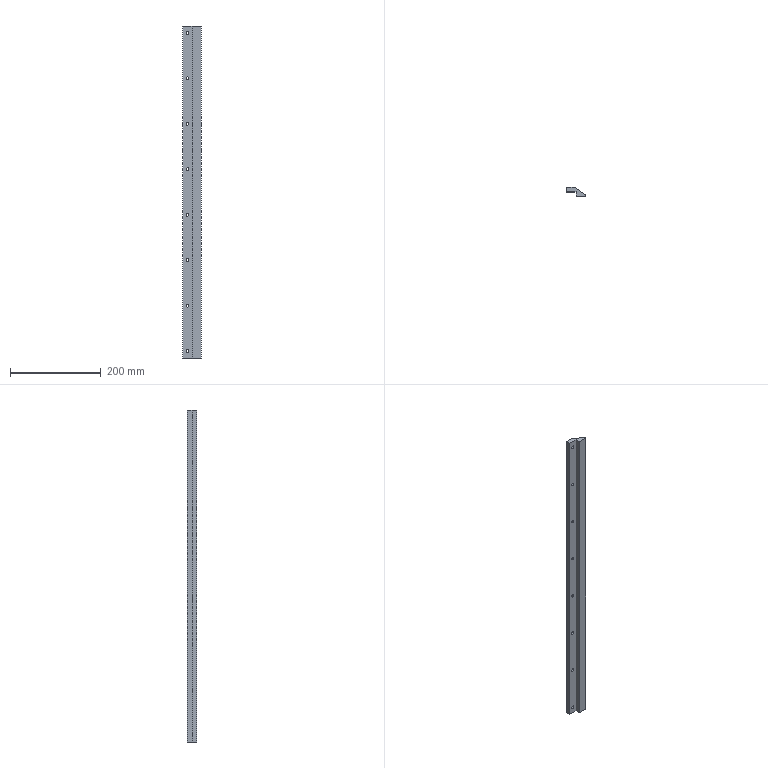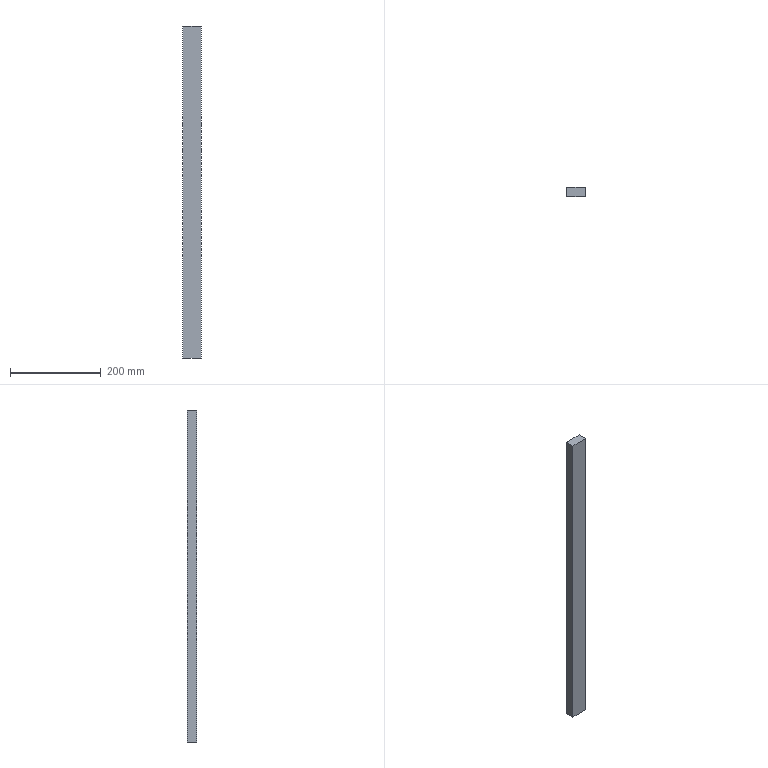CAM job | NX | 3+2 milling, drilling | part box 40 x 20 x 730 mm | stock box 40 x 20 x 730 mm
Tools:
number,name,description,diameter,corner_radius,flute_length,length,flutes
15,D10,Milling Tool-5 Parameters,10.0,0.0,50.0,75.0,2
14,D10JING,Milling Tool-5 Parameters,10.0,0.0,50.0,75.0,2
1,D6A45,Milling Tool-5 Parameters,6.0,0.0,50.0,75.0,2
16,6.2ZT,Drilling Tool,6.2,0.0,35.0,50.0,2
16,D6R0.5,Milling Tool-5 Parameters,6.0,0.5,50.0,75.0,2
Operations:
program,operation,operation_type,tool,method,geometry_group,spindle_rpm,surface_speed,feed_per_tooth,feed_cut,feed_plunge,cut_length_mm,path_length_mm,cut_time_min,machine_time_min
1,FLOOR_WALL_1,VolumeBased25DMillingOperation,D10,METHOD,A,9500.0,298.0,0.1579,3000.0,100.0,29416.226,29611.431,9.805,9.825
1,FLOOR_WALL_1_COPY,VolumeBased25DMillingOperation,D10JING,METHOD,A,9500.0,298.0,0.0789,1500.0,100.0,3727.758,3806.258,2.485,2.493
1,DRILLING,Operation,D6A45,METHOD,A,9500.0,179.0,0.0132,250.0,0.0,32.0,865.315,0.128,0.2113
1,DRILLING_COPY_COPY,Operation,6.2ZT,METHOD,A,2000.0,21.0,0.0375,150.0,0.0,130.901,1063.118,0.8727,0.9659
1,PLANAR_MILL,PlanarMilling,D6A45,METHOD,A,9500.0,179.0,0.0658,1250.0,100.0,735.094,794.094,0.5881,0.594
1,PLANAR_MILL_COPY,PlanarMilling,D6A45,METHOD,A,9500.0,179.0,0.0658,1250.0,100.0,938.204,3077.585,0.7506,0.9645
2,ZLEVEL_PROFILE,ZLevelMilling,D10,METHOD,B,9500.0,298.0,0.1053,2000.0,1000.0,36342.479,36424.253,18.173,18.181
2,ZLEVEL_PROFILE_COPY,ZLevelMilling,D6R0.5,METHOD,B,9500.0,119.0,0.1316,2500.0,1000.0,176695.495,176777.195,70.68,70.688